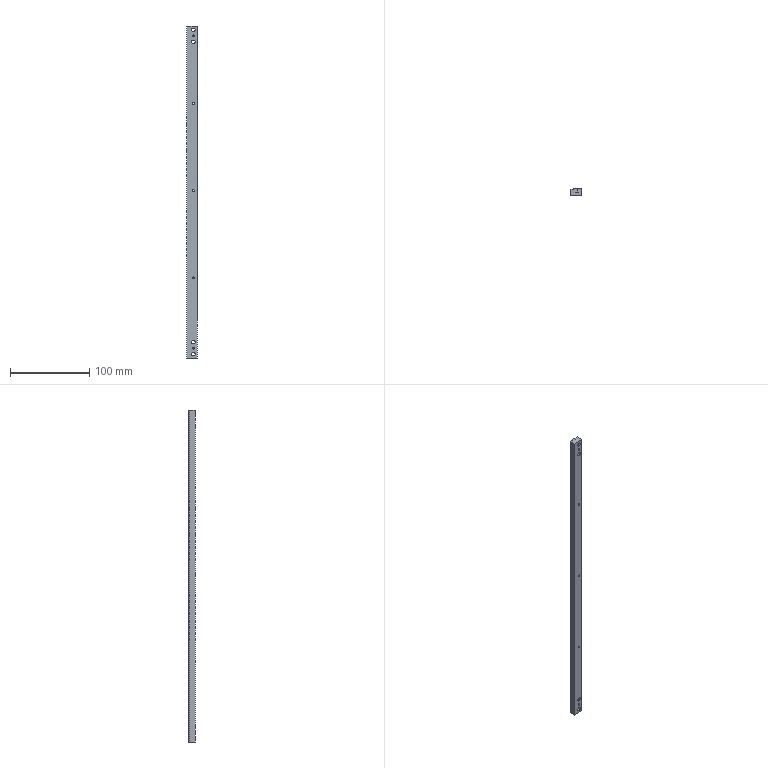Part | STEP file | 11-FG-B00611 | 1 solid | 47 faces | box 13.5 x 8.4 x 419 mm | volume 44557 mm3 | cylinder 30 | plane 13 | cone 4 | commonest cylinder face diameters 2.5 x14 4.5 x8 8 x8
STEP:
#1=CARTESIAN_POINT('',(8.5,0.,209.75));
#2=VERTEX_POINT('',#1);
#3=CARTESIAN_POINT('',(8.5,0.,212.25));
#4=VERTEX_POINT('',#3);
#5=CARTESIAN_POINT('',(8.5,0.,211.));
#6=DIRECTION('',(0.,1.,0.));
#7=DIRECTION('',(0.,0.,1.));
#8=AXIS2_PLACEMENT_3D('',#5,#6,#7);
#9=CIRCLE('',#8,1.25);
#10=EDGE_CURVE('',#2,#4,#9,.T.);
#11=ORIENTED_EDGE('',*,*,#10,.F.);
#12=CARTESIAN_POINT('',(8.5,8.4,209.75));
#13=VERTEX_POINT('',#12);
#14=CARTESIAN_POINT('',(8.5,8.,209.75));
#15=DIRECTION('',(0.,1.,0.));
#16=VECTOR('',#15,1000.);
#17=LINE('',#14,#16);
#18=EDGE_CURVE('',#2,#13,#17,.T.);
#19=ORIENTED_EDGE('',*,*,#18,.T.);
#20=CARTESIAN_POINT('',(8.5,8.4,212.25));
#21=VERTEX_POINT('',#20);
#22=CARTESIAN_POINT('',(8.5,8.4,211.));
#23=DIRECTION('',(0.,1.,0.));
#24=DIRECTION('',(0.,0.,-1.));
#25=AXIS2_PLACEMENT_3D('',#22,#23,#24);
#26=CIRCLE('',#25,1.25);
#27=EDGE_CURVE('',#13,#21,#26,.T.);
#28=ORIENTED_EDGE('',*,*,#27,.T.);
#29=CARTESIAN_POINT('',(8.5,8.,212.25));
#30=DIRECTION('',(0.,1.,0.));
#31=VECTOR('',#30,1000.);
#32=LINE('',#29,#31);
#33=EDGE_CURVE('',#4,#21,#32,.T.);
#34=ORIENTED_EDGE('',*,*,#33,.F.);
#35=EDGE_LOOP('',(#11,#19,#28,#34));
#36=FACE_OUTER_BOUND('',#35,.T.);
#37=CARTESIAN_POINT('',(8.5,8.,211.));
#38=DIRECTION('',(0.,1.,0.));
#39=DIRECTION('',(0.,0.,1.));
#40=AXIS2_PLACEMENT_3D('',#37,#38,#39);
#41=CYLINDRICAL_SURFACE('',#40,1.25);
#42=ADVANCED_FACE('',(#36),#41,.F.);
#43=CARTESIAN_POINT('',(8.5,0.,319.75));
#44=VERTEX_POINT('',#43);
#45=CARTESIAN_POINT('',(8.5,0.,322.25));
#46=VERTEX_POINT('',#45);
#47=CARTESIAN_POINT('',(8.5,0.,321.));
#48=DIRECTION('',(0.,1.,0.));
#49=DIRECTION('',(0.,0.,1.));
#50=AXIS2_PLACEMENT_3D('',#47,#48,#49);
#51=CIRCLE('',#50,1.25);
#52=EDGE_CURVE('',#44,#46,#51,.T.);
#53=ORIENTED_EDGE('',*,*,#52,.F.);
#54=CARTESIAN_POINT('',(8.5,8.4,319.75));
#55=VERTEX_POINT('',#54);
#56=CARTESIAN_POINT('',(8.5,8.,319.75));
#57=DIRECTION('',(0.,1.,0.));
#58=VECTOR('',#57,1000.);
#59=LINE('',#56,#58);
#60=EDGE_CURVE('',#44,#55,#59,.T.);
#61=ORIENTED_EDGE('',*,*,#60,.T.);
#62=CARTESIAN_POINT('',(8.5,8.4,322.25));
#63=VERTEX_POINT('',#62);
#64=CARTESIAN_POINT('',(8.5,8.4,321.));
#65=DIRECTION('',(0.,1.,0.));
#66=DIRECTION('',(0.,0.,-1.));
#67=AXIS2_PLACEMENT_3D('',#64,#65,#66);
#68=CIRCLE('',#67,1.25);
#69=EDGE_CURVE('',#55,#63,#68,.T.);
#70=ORIENTED_EDGE('',*,*,#69,.T.);
#71=CARTESIAN_POINT('',(8.5,8.,322.25));
#72=DIRECTION('',(0.,1.,0.));
#73=VECTOR('',#72,1000.);
#74=LINE('',#71,#73);
#75=EDGE_CURVE('',#46,#63,#74,.T.);
#76=ORIENTED_EDGE('',*,*,#75,.F.);
#77=EDGE_LOOP('',(#53,#61,#70,#76));
#78=FACE_OUTER_BOUND('',#77,.T.);
#79=CARTESIAN_POINT('',(8.5,8.,321.));
#80=DIRECTION('',(0.,1.,0.));
#81=DIRECTION('',(0.,0.,1.));
#82=AXIS2_PLACEMENT_3D('',#79,#80,#81);
#83=CYLINDRICAL_SURFACE('',#82,1.25);
#84=ADVANCED_FACE('',(#78),#83,.F.);
#85=CARTESIAN_POINT('',(8.5,0.,99.75));
#86=VERTEX_POINT('',#85);
#87=CARTESIAN_POINT('',(8.5,0.,102.25));
#88=VERTEX_POINT('',#87);
#89=CARTESIAN_POINT('',(8.5,0.,101.));
#90=DIRECTION('',(0.,1.,0.));
#91=DIRECTION('',(0.,0.,1.));
#92=AXIS2_PLACEMENT_3D('',#89,#90,#91);
#93=CIRCLE('',#92,1.25);
#94=EDGE_CURVE('',#86,#88,#93,.T.);
#95=ORIENTED_EDGE('',*,*,#94,.F.);
#96=CARTESIAN_POINT('',(8.5,8.4,99.75));
#97=VERTEX_POINT('',#96);
#98=CARTESIAN_POINT('',(8.5,8.,99.75));
#99=DIRECTION('',(0.,1.,0.));
#100=VECTOR('',#99,1000.);
#101=LINE('',#98,#100);
#102=EDGE_CURVE('',#86,#97,#101,.T.);
#103=ORIENTED_EDGE('',*,*,#102,.T.);
#104=CARTESIAN_POINT('',(8.5,8.4,102.25));
#105=VERTEX_POINT('',#104);
#106=CARTESIAN_POINT('',(8.5,8.4,101.));
#107=DIRECTION('',(0.,1.,0.));
#108=DIRECTION('',(0.,0.,-1.));
#109=AXIS2_PLACEMENT_3D('',#106,#107,#108);
#110=CIRCLE('',#109,1.25);
#111=EDGE_CURVE('',#97,#105,#110,.T.);
#112=ORIENTED_EDGE('',*,*,#111,.T.);
#113=CARTESIAN_POINT('',(8.5,8.,102.25));
#114=DIRECTION('',(0.,1.,0.));
#115=VECTOR('',#114,1000.);
#116=LINE('',#113,#115);
#117=EDGE_CURVE('',#88,#105,#116,.T.);
#118=ORIENTED_EDGE('',*,*,#117,.F.);
#119=EDGE_LOOP('',(#95,#103,#112,#118));
#120=FACE_OUTER_BOUND('',#119,.T.);
#121=CARTESIAN_POINT('',(8.5,8.,101.));
#122=DIRECTION('',(0.,1.,0.));
#123=DIRECTION('',(0.,0.,1.));
#124=AXIS2_PLACEMENT_3D('',#121,#122,#123);
#125=CYLINDRICAL_SURFACE('',#124,1.25);
#126=ADVANCED_FACE('',(#120),#125,.F.);
#127=CARTESIAN_POINT('',(8.5,0.,11.25));
#128=VERTEX_POINT('',#127);
#129=CARTESIAN_POINT('',(8.5,0.,13.75));
#130=VERTEX_POINT('',#129);
#131=CARTESIAN_POINT('',(8.5,0.,12.5));
#132=DIRECTION('',(0.,1.,0.));
#133=DIRECTION('',(0.,0.,1.));
#134=AXIS2_PLACEMENT_3D('',#131,#132,#133);
#135=CIRCLE('',#134,1.25);
#136=EDGE_CURVE('',#128,#130,#135,.T.);
#137=ORIENTED_EDGE('',*,*,#136,.F.);
#138=CARTESIAN_POINT('',(8.5,8.4,11.25));
#139=VERTEX_POINT('',#138);
#140=CARTESIAN_POINT('',(8.5,8.,11.25));
#141=DIRECTION('',(0.,1.,0.));
#142=VECTOR('',#141,1000.);
#143=LINE('',#140,#142);
#144=EDGE_CURVE('',#128,#139,#143,.T.);
#145=ORIENTED_EDGE('',*,*,#144,.T.);
#146=CARTESIAN_POINT('',(8.5,8.4,13.75));
#147=VERTEX_POINT('',#146);
#148=CARTESIAN_POINT('',(8.5,8.4,12.5));
#149=DIRECTION('',(0.,1.,0.));
#150=DIRECTION('',(0.,0.,-1.));
#151=AXIS2_PLACEMENT_3D('',#148,#149,#150);
#152=CIRCLE('',#151,1.25);
#153=EDGE_CURVE('',#139,#147,#152,.T.);
#154=ORIENTED_EDGE('',*,*,#153,.T.);
#155=CARTESIAN_POINT('',(8.5,8.,13.75));
#156=DIRECTION('',(0.,1.,0.));
#157=VECTOR('',#156,1000.);
#158=LINE('',#155,#157);
#159=EDGE_CURVE('',#130,#147,#158,.T.);
#160=ORIENTED_EDGE('',*,*,#159,.F.);
#161=EDGE_LOOP('',(#137,#145,#154,#160));
#162=FACE_OUTER_BOUND('',#161,.T.);
#163=CARTESIAN_POINT('',(8.5,8.,12.5));
#164=DIRECTION('',(0.,1.,0.));
#165=DIRECTION('',(0.,0.,1.));
#166=AXIS2_PLACEMENT_3D('',#163,#164,#165);
#167=CYLINDRICAL_SURFACE('',#166,1.25);
#168=ADVANCED_FACE('',(#162),#167,.F.);
#169=CARTESIAN_POINT('',(8.5,0.,405.25));
#170=VERTEX_POINT('',#169);
#171=CARTESIAN_POINT('',(8.5,0.,407.75));
#172=VERTEX_POINT('',#171);
#173=CARTESIAN_POINT('',(8.5,0.,406.5));
#174=DIRECTION('',(0.,1.,0.));
#175=DIRECTION('',(0.,0.,1.));
#176=AXIS2_PLACEMENT_3D('',#173,#174,#175);
#177=CIRCLE('',#176,1.25);
#178=EDGE_CURVE('',#170,#172,#177,.T.);
#179=ORIENTED_EDGE('',*,*,#178,.F.);
#180=CARTESIAN_POINT('',(8.5,8.4,405.25));
#181=VERTEX_POINT('',#180);
#182=CARTESIAN_POINT('',(8.5,8.,405.25));
#183=DIRECTION('',(0.,1.,0.));
#184=VECTOR('',#183,1000.);
#185=LINE('',#182,#184);
#186=EDGE_CURVE('',#170,#181,#185,.T.);
#187=ORIENTED_EDGE('',*,*,#186,.T.);
#188=CARTESIAN_POINT('',(8.5,8.4,407.75));
#189=VERTEX_POINT('',#188);
#190=CARTESIAN_POINT('',(8.5,8.4,406.5));
#191=DIRECTION('',(0.,1.,0.));
#192=DIRECTION('',(0.,0.,-1.));
#193=AXIS2_PLACEMENT_3D('',#190,#191,#192);
#194=CIRCLE('',#193,1.25);
#195=EDGE_CURVE('',#181,#189,#194,.T.);
#196=ORIENTED_EDGE('',*,*,#195,.T.);
#197=CARTESIAN_POINT('',(8.5,8.,407.75));
#198=DIRECTION('',(0.,1.,0.));
#199=VECTOR('',#198,1000.);
#200=LINE('',#197,#199);
#201=EDGE_CURVE('',#172,#189,#200,.T.);
#202=ORIENTED_EDGE('',*,*,#201,.F.);
#203=EDGE_LOOP('',(#179,#187,#196,#202));
#204=FACE_OUTER_BOUND('',#203,.T.);
#205=CARTESIAN_POINT('',(8.5,8.,406.5));
#206=DIRECTION('',(0.,1.,0.));
#207=DIRECTION('',(0.,0.,1.));
#208=AXIS2_PLACEMENT_3D('',#205,#206,#207);
#209=CYLINDRICAL_SURFACE('',#208,1.25);
#210=ADVANCED_FACE('',(#204),#209,.F.);
#211=CARTESIAN_POINT('',(8.5,3.6,410.));
#212=VERTEX_POINT('',#211);
#213=CARTESIAN_POINT('',(8.5,3.6,418.));
#214=VERTEX_POINT('',#213);
#215=CARTESIAN_POINT('',(8.5,3.6,414.));
#216=DIRECTION('',(0.,1.,0.));
#217=DIRECTION('',(0.,0.,1.));
#218=AXIS2_PLACEMENT_3D('',#215,#216,#217);
#219=CIRCLE('',#218,4.);
#220=EDGE_CURVE('',#212,#214,#219,.T.);
#221=ORIENTED_EDGE('',*,*,#220,.F.);
#222=CARTESIAN_POINT('',(8.5,8.4,410.));
#223=VERTEX_POINT('',#222);
#224=CARTESIAN_POINT('',(8.5,8.,410.));
#225=DIRECTION('',(0.,1.,0.));
#226=VECTOR('',#225,1000.);
#227=LINE('',#224,#226);
#228=EDGE_CURVE('',#212,#223,#227,.T.);
#229=ORIENTED_EDGE('',*,*,#228,.T.);
#230=CARTESIAN_POINT('',(8.5,8.4,418.));
#231=VERTEX_POINT('',#230);
#232=CARTESIAN_POINT('',(8.5,8.4,414.));
#233=DIRECTION('',(0.,1.,0.));
#234=DIRECTION('',(0.,0.,-1.));
#235=AXIS2_PLACEMENT_3D('',#232,#233,#234);
#236=CIRCLE('',#235,4.);
#237=EDGE_CURVE('',#223,#231,#236,.T.);
#238=ORIENTED_EDGE('',*,*,#237,.T.);
#239=CARTESIAN_POINT('',(8.5,8.,418.));
#240=DIRECTION('',(0.,1.,0.));
#241=VECTOR('',#240,1000.);
#242=LINE('',#239,#241);
#243=EDGE_CURVE('',#214,#231,#242,.T.);
#244=ORIENTED_EDGE('',*,*,#243,.F.);
#245=EDGE_LOOP('',(#221,#229,#238,#244));
#246=FACE_OUTER_BOUND('',#245,.T.);
#247=CARTESIAN_POINT('',(8.5,8.,414.));
#248=DIRECTION('',(0.,1.,0.));
#249=DIRECTION('',(0.,0.,1.));
#250=AXIS2_PLACEMENT_3D('',#247,#248,#249);
#251=CYLINDRICAL_SURFACE('',#250,4.);
#252=ADVANCED_FACE('',(#246),#251,.F.);
#253=CARTESIAN_POINT('',(8.5,0.,411.75));
#254=VERTEX_POINT('',#253);
#255=CARTESIAN_POINT('',(8.5,0.,416.25));
#256=VERTEX_POINT('',#255);
#257=CARTESIAN_POINT('',(8.5,0.,414.));
#258=DIRECTION('',(0.,1.,0.));
#259=DIRECTION('',(0.,0.,1.));
#260=AXIS2_PLACEMENT_3D('',#257,#258,#259);
#261=CIRCLE('',#260,2.25);
#262=EDGE_CURVE('',#254,#256,#261,.T.);
#263=ORIENTED_EDGE('',*,*,#262,.F.);
#264=CARTESIAN_POINT('',(8.5,3.6,411.75));
#265=VERTEX_POINT('',#264);
#266=CARTESIAN_POINT('',(8.5,8.,411.75));
#267=DIRECTION('',(0.,1.,0.));
#268=VECTOR('',#267,1000.);
#269=LINE('',#266,#268);
#270=EDGE_CURVE('',#254,#265,#269,.T.);
#271=ORIENTED_EDGE('',*,*,#270,.T.);
#272=CARTESIAN_POINT('',(8.5,3.6,416.25));
#273=VERTEX_POINT('',#272);
#274=CARTESIAN_POINT('',(8.5,3.6,414.));
#275=DIRECTION('',(0.,1.,0.));
#276=DIRECTION('',(0.,0.,1.));
#277=AXIS2_PLACEMENT_3D('',#274,#275,#276);
#278=CIRCLE('',#277,2.25);
#279=EDGE_CURVE('',#265,#273,#278,.T.);
#280=ORIENTED_EDGE('',*,*,#279,.T.);
#281=CARTESIAN_POINT('',(8.5,8.,416.25));
#282=DIRECTION('',(0.,1.,0.));
#283=VECTOR('',#282,1000.);
#284=LINE('',#281,#283);
#285=EDGE_CURVE('',#256,#273,#284,.T.);
#286=ORIENTED_EDGE('',*,*,#285,.F.);
#287=EDGE_LOOP('',(#263,#271,#280,#286));
#288=FACE_OUTER_BOUND('',#287,.T.);
#289=CARTESIAN_POINT('',(8.5,8.,414.));
#290=DIRECTION('',(0.,1.,0.));
#291=DIRECTION('',(0.,0.,1.));
#292=AXIS2_PLACEMENT_3D('',#289,#290,#291);
#293=CYLINDRICAL_SURFACE('',#292,2.25);
#294=ADVANCED_FACE('',(#288),#293,.F.);
#295=CARTESIAN_POINT('',(8.5,3.6,395.));
#296=VERTEX_POINT('',#295);
#297=CARTESIAN_POINT('',(8.5,3.6,403.));
#298=VERTEX_POINT('',#297);
#299=CARTESIAN_POINT('',(8.5,3.6,399.));
#300=DIRECTION('',(0.,1.,0.));
#301=DIRECTION('',(0.,0.,1.));
#302=AXIS2_PLACEMENT_3D('',#299,#300,#301);
#303=CIRCLE('',#302,4.);
#304=EDGE_CURVE('',#296,#298,#303,.T.);
#305=ORIENTED_EDGE('',*,*,#304,.F.);
#306=CARTESIAN_POINT('',(8.5,8.4,395.));
#307=VERTEX_POINT('',#306);
#308=CARTESIAN_POINT('',(8.5,8.,395.));
#309=DIRECTION('',(0.,1.,0.));
#310=VECTOR('',#309,1000.);
#311=LINE('',#308,#310);
#312=EDGE_CURVE('',#296,#307,#311,.T.);
#313=ORIENTED_EDGE('',*,*,#312,.T.);
#314=CARTESIAN_POINT('',(8.5,8.4,403.));
#315=VERTEX_POINT('',#314);
#316=CARTESIAN_POINT('',(8.5,8.4,399.));
#317=DIRECTION('',(0.,1.,0.));
#318=DIRECTION('',(0.,0.,-1.));
#319=AXIS2_PLACEMENT_3D('',#316,#317,#318);
#320=CIRCLE('',#319,4.);
#321=EDGE_CURVE('',#307,#315,#320,.T.);
#322=ORIENTED_EDGE('',*,*,#321,.T.);
#323=CARTESIAN_POINT('',(8.5,8.,403.));
#324=DIRECTION('',(0.,1.,0.));
#325=VECTOR('',#324,1000.);
#326=LINE('',#323,#325);
#327=EDGE_CURVE('',#298,#315,#326,.T.);
#328=ORIENTED_EDGE('',*,*,#327,.F.);
#329=EDGE_LOOP('',(#305,#313,#322,#328));
#330=FACE_OUTER_BOUND('',#329,.T.);
#331=CARTESIAN_POINT('',(8.5,8.,399.));
#332=DIRECTION('',(0.,1.,0.));
#333=DIRECTION('',(0.,0.,1.));
#334=AXIS2_PLACEMENT_3D('',#331,#332,#333);
#335=CYLINDRICAL_SURFACE('',#334,4.);
#336=ADVANCED_FACE('',(#330),#335,.F.);
#337=CARTESIAN_POINT('',(8.5,0.,396.75));
#338=VERTEX_POINT('',#337);
#339=CARTESIAN_POINT('',(8.5,0.,401.25));
#340=VERTEX_POINT('',#339);
#341=CARTESIAN_POINT('',(8.5,0.,399.));
#342=DIRECTION('',(0.,1.,0.));
#343=DIRECTION('',(0.,0.,1.));
#344=AXIS2_PLACEMENT_3D('',#341,#342,#343);
#345=CIRCLE('',#344,2.25);
#346=EDGE_CURVE('',#338,#340,#345,.T.);
#347=ORIENTED_EDGE('',*,*,#346,.F.);
#348=CARTESIAN_POINT('',(8.5,3.6,396.75));
#349=VERTEX_POINT('',#348);
#350=CARTESIAN_POINT('',(8.5,8.,396.75));
#351=DIRECTION('',(0.,1.,0.));
#352=VECTOR('',#351,1000.);
#353=LINE('',#350,#352);
#354=EDGE_CURVE('',#338,#349,#353,.T.);
#355=ORIENTED_EDGE('',*,*,#354,.T.);
#356=CARTESIAN_POINT('',(8.5,3.6,401.25));
#357=VERTEX_POINT('',#356);
#358=CARTESIAN_POINT('',(8.5,3.6,399.));
#359=DIRECTION('',(0.,1.,0.));
#360=DIRECTION('',(0.,0.,1.));
#361=AXIS2_PLACEMENT_3D('',#358,#359,#360);
#362=CIRCLE('',#361,2.25);
#363=EDGE_CURVE('',#349,#357,#362,.T.);
#364=ORIENTED_EDGE('',*,*,#363,.T.);
#365=CARTESIAN_POINT('',(8.5,8.,401.25));
#366=DIRECTION('',(0.,1.,0.));
#367=VECTOR('',#366,1000.);
#368=LINE('',#365,#367);
#369=EDGE_CURVE('',#340,#357,#368,.T.);
#370=ORIENTED_EDGE('',*,*,#369,.F.);
#371=EDGE_LOOP('',(#347,#355,#364,#370));
#372=FACE_OUTER_BOUND('',#371,.T.);
#373=CARTESIAN_POINT('',(8.5,8.,399.));
#374=DIRECTION('',(0.,1.,0.));
#375=DIRECTION('',(0.,0.,1.));
#376=AXIS2_PLACEMENT_3D('',#373,#374,#375);
#377=CYLINDRICAL_SURFACE('',#376,2.25);
#378=ADVANCED_FACE('',(#372),#377,.F.);
#379=CARTESIAN_POINT('',(6.,4.,49.75));
#380=VERTEX_POINT('',#379);
#381=CARTESIAN_POINT('',(6.,4.,47.25));
#382=VERTEX_POINT('',#381);
#383=CARTESIAN_POINT('',(6.,4.,48.5));
#384=DIRECTION('',(1.,0.,0.));
#385=DIRECTION('',(0.,0.,-1.));
#386=AXIS2_PLACEMENT_3D('',#383,#384,#385);
#387=CIRCLE('',#386,1.25);
#388=EDGE_CURVE('',#380,#382,#387,.T.);
#389=ORIENTED_EDGE('',*,*,#388,.F.);
#390=CARTESIAN_POINT('',(13.5,4.,49.75));
#391=VERTEX_POINT('',#390);
#392=CARTESIAN_POINT('',(13.5,4.,49.75));
#393=DIRECTION('',(1.,0.,0.));
#394=VECTOR('',#393,1000.);
#395=LINE('',#392,#394);
#396=EDGE_CURVE('',#380,#391,#395,.T.);
#397=ORIENTED_EDGE('',*,*,#396,.T.);
#398=CARTESIAN_POINT('',(13.5,4.,47.25));
#399=VERTEX_POINT('',#398);
#400=CARTESIAN_POINT('',(13.5,4.,48.5));
#401=DIRECTION('',(1.,0.,0.));
#402=DIRECTION('',(0.,0.,-1.));
#403=AXIS2_PLACEMENT_3D('',#400,#401,#402);
#404=CIRCLE('',#403,1.25);
#405=EDGE_CURVE('',#391,#399,#404,.T.);
#406=ORIENTED_EDGE('',*,*,#405,.T.);
#407=CARTESIAN_POINT('',(13.5,4.,47.25));
#408=DIRECTION('',(1.,0.,0.));
#409=VECTOR('',#408,1000.);
#410=LINE('',#407,#409);
#411=EDGE_CURVE('',#382,#399,#410,.T.);
#412=ORIENTED_EDGE('',*,*,#411,.F.);
#413=EDGE_LOOP('',(#389,#397,#406,#412));
#414=FACE_OUTER_BOUND('',#413,.T.);
#415=CARTESIAN_POINT('',(13.5,4.,48.5));
#416=DIRECTION('',(1.,0.,0.));
#417=DIRECTION('',(0.,0.,-1.));
#418=AXIS2_PLACEMENT_3D('',#415,#416,#417);
#419=CYLINDRICAL_SURFACE('',#418,1.25);
#420=ADVANCED_FACE('',(#414),#419,.F.);
#421=CARTESIAN_POINT('',(5.249,4.,48.5));
#422=VERTEX_POINT('',#421);
#423=CARTESIAN_POINT('',(6.,4.,47.25));
#424=DIRECTION('',(0.515,0.,-0.8572));
#425=VECTOR('',#424,1000.);
#426=LINE('',#423,#425);
#427=EDGE_CURVE('',#422,#382,#426,.T.);
#428=ORIENTED_EDGE('',*,*,#427,.F.);
#429=CARTESIAN_POINT('',(6.,4.,49.75));
#430=DIRECTION('',(0.515,0.,0.8572));
#431=VECTOR('',#430,1000.);
#432=LINE('',#429,#431);
#433=EDGE_CURVE('',#422,#380,#432,.T.);
#434=ORIENTED_EDGE('',*,*,#433,.T.);
#435=ORIENTED_EDGE('',*,*,#388,.T.);
#436=EDGE_LOOP('',(#428,#434,#435));
#437=FACE_OUTER_BOUND('',#436,.T.);
#438=CARTESIAN_POINT('',(6.,4.,48.5));
#439=DIRECTION('',(1.,0.,0.));
#440=DIRECTION('',(0.,0.,-1.));
#441=AXIS2_PLACEMENT_3D('',#438,#439,#440);
#442=CONICAL_SURFACE('',#441,1.25,1.03);
#443=ADVANCED_FACE('',(#437),#442,.F.);
#444=CARTESIAN_POINT('',(6.,4.,42.75));
#445=VERTEX_POINT('',#444);
#446=CARTESIAN_POINT('',(6.,4.,40.25));
#447=VERTEX_POINT('',#446);
#448=CARTESIAN_POINT('',(6.,4.,41.5));
#449=DIRECTION('',(1.,0.,0.));
#450=DIRECTION('',(0.,0.,-1.));
#451=AXIS2_PLACEMENT_3D('',#448,#449,#450);
#452=CIRCLE('',#451,1.25);
#453=EDGE_CURVE('',#445,#447,#452,.T.);
#454=ORIENTED_EDGE('',*,*,#453,.F.);
#455=CARTESIAN_POINT('',(13.5,4.,42.75));
#456=VERTEX_POINT('',#455);
#457=CARTESIAN_POINT('',(13.5,4.,42.75));
#458=DIRECTION('',(1.,0.,0.));
#459=VECTOR('',#458,1000.);
#460=LINE('',#457,#459);
#461=EDGE_CURVE('',#445,#456,#460,.T.);
#462=ORIENTED_EDGE('',*,*,#461,.T.);
#463=CARTESIAN_POINT('',(13.5,4.,40.25));
#464=VERTEX_POINT('',#463);
#465=CARTESIAN_POINT('',(13.5,4.,41.5));
#466=DIRECTION('',(1.,0.,0.));
#467=DIRECTION('',(0.,0.,-1.));
#468=AXIS2_PLACEMENT_3D('',#465,#466,#467);
#469=CIRCLE('',#468,1.25);
#470=EDGE_CURVE('',#456,#464,#469,.T.);
#471=ORIENTED_EDGE('',*,*,#470,.T.);
#472=CARTESIAN_POINT('',(13.5,4.,40.25));
#473=DIRECTION('',(1.,0.,0.));
#474=VECTOR('',#473,1000.);
#475=LINE('',#472,#474);
#476=EDGE_CURVE('',#447,#464,#475,.T.);
#477=ORIENTED_EDGE('',*,*,#476,.F.);
#478=EDGE_LOOP('',(#454,#462,#471,#477));
#479=FACE_OUTER_BOUND('',#478,.T.);
#480=CARTESIAN_POINT('',(13.5,4.,41.5));
#481=DIRECTION('',(1.,0.,0.));
#482=DIRECTION('',(0.,0.,-1.));
#483=AXIS2_PLACEMENT_3D('',#480,#481,#482);
#484=CYLINDRICAL_SURFACE('',#483,1.25);
#485=ADVANCED_FACE('',(#479),#484,.F.);
#486=CARTESIAN_POINT('',(5.249,4.,41.5));
#487=VERTEX_POINT('',#486);
#488=CARTESIAN_POINT('',(6.,4.,40.25));
#489=DIRECTION('',(0.515,0.,-0.8572));
#490=VECTOR('',#489,1000.);
#491=LINE('',#488,#490);
#492=EDGE_CURVE('',#487,#447,#491,.T.);
#493=ORIENTED_EDGE('',*,*,#492,.F.);
#494=CARTESIAN_POINT('',(6.,4.,42.75));
#495=DIRECTION('',(0.515,0.,0.8572));
#496=VECTOR('',#495,1000.);
#497=LINE('',#494,#496);
#498=EDGE_CURVE('',#487,#445,#497,.T.);
#499=ORIENTED_EDGE('',*,*,#498,.T.);
#500=ORIENTED_EDGE('',*,*,#453,.T.);
#501=EDGE_LOOP('',(#493,#499,#500));
#502=FACE_OUTER_BOUND('',#501,.T.);
#503=CARTESIAN_POINT('',(6.,4.,41.5));
#504=DIRECTION('',(1.,0.,0.));
#505=DIRECTION('',(0.,0.,-1.));
#506=AXIS2_PLACEMENT_3D('',#503,#504,#505);
#507=CONICAL_SURFACE('',#506,1.25,1.03);
#508=ADVANCED_FACE('',(#502),#507,.F.);
#509=CARTESIAN_POINT('',(8.5,3.4,16.));
#510=VERTEX_POINT('',#509);
#511=CARTESIAN_POINT('',(8.5,3.4,24.));
#512=VERTEX_POINT('',#511);
#513=CARTESIAN_POINT('',(8.5,3.4,20.));
#514=DIRECTION('',(0.,1.,0.));
#515=DIRECTION('',(0.,0.,1.));
#516=AXIS2_PLACEMENT_3D('',#513,#514,#515);
#517=CIRCLE('',#516,4.);
#518=EDGE_CURVE('',#510,#512,#517,.T.);
#519=ORIENTED_EDGE('',*,*,#518,.F.);
#520=CARTESIAN_POINT('',(8.5,8.4,16.));
#521=VERTEX_POINT('',#520);
#522=CARTESIAN_POINT('',(8.5,8.,16.));
#523=DIRECTION('',(0.,1.,0.));
#524=VECTOR('',#523,1000.);
#525=LINE('',#522,#524);
#526=EDGE_CURVE('',#510,#521,#525,.T.);
#527=ORIENTED_EDGE('',*,*,#526,.T.);
#528=CARTESIAN_POINT('',(8.5,8.4,24.));
#529=VERTEX_POINT('',#528);
#530=CARTESIAN_POINT('',(8.5,8.4,20.));
#531=DIRECTION('',(0.,1.,0.));
#532=DIRECTION('',(0.,0.,-1.));
#533=AXIS2_PLACEMENT_3D('',#530,#531,#532);
#534=CIRCLE('',#533,4.);
#535=EDGE_CURVE('',#521,#529,#534,.T.);
#536=ORIENTED_EDGE('',*,*,#535,.T.);
#537=CARTESIAN_POINT('',(8.5,8.,24.));
#538=DIRECTION('',(0.,1.,0.));
#539=VECTOR('',#538,1000.);
#540=LINE('',#537,#539);
#541=EDGE_CURVE('',#512,#529,#540,.T.);
#542=ORIENTED_EDGE('',*,*,#541,.F.);
#543=EDGE_LOOP('',(#519,#527,#536,#542));
#544=FACE_OUTER_BOUND('',#543,.T.);
#545=CARTESIAN_POINT('',(8.5,8.,20.));
#546=DIRECTION('',(0.,1.,0.));
#547=DIRECTION('',(0.,0.,1.));
#548=AXIS2_PLACEMENT_3D('',#545,#546,#547);
#549=CYLINDRICAL_SURFACE('',#548,4.);
#550=ADVANCED_FACE('',(#544),#549,.F.);
#551=CARTESIAN_POINT('',(8.5,0.,17.75));
#552=VERTEX_POINT('',#551);
#553=CARTESIAN_POINT('',(8.5,0.,22.25));
#554=VERTEX_POINT('',#553);
#555=CARTESIAN_POINT('',(8.5,0.,20.));
#556=DIRECTION('',(0.,1.,0.));
#557=DIRECTION('',(0.,0.,1.));
#558=AXIS2_PLACEMENT_3D('',#555,#556,#557);
#559=CIRCLE('',#558,2.25);
#560=EDGE_CURVE('',#552,#554,#559,.T.);
#561=ORIENTED_EDGE('',*,*,#560,.F.);
#562=CARTESIAN_POINT('',(8.5,3.4,17.75));
#563=VERTEX_POINT('',#562);
#564=CARTESIAN_POINT('',(8.5,8.,17.75));
#565=DIRECTION('',(0.,1.,0.));
#566=VECTOR('',#565,1000.);
#567=LINE('',#564,#566);
#568=EDGE_CURVE('',#552,#563,#567,.T.);
#569=ORIENTED_EDGE('',*,*,#568,.T.);
#570=CARTESIAN_POINT('',(8.5,3.4,22.25));
#571=VERTEX_POINT('',#570);
#572=CARTESIAN_POINT('',(8.5,3.4,20.));
#573=DIRECTION('',(0.,1.,0.));
#574=DIRECTION('',(0.,0.,1.));
#575=AXIS2_PLACEMENT_3D('',#572,#573,#574);
#576=CIRCLE('',#575,2.25);
#577=EDGE_CURVE('',#563,#571,#576,.T.);
#578=ORIENTED_EDGE('',*,*,#577,.T.);
#579=CARTESIAN_POINT('',(8.5,8.,22.25));
#580=DIRECTION('',(0.,1.,0.));
#581=VECTOR('',#580,1000.);
#582=LINE('',#579,#581);
#583=EDGE_CURVE('',#554,#571,#582,.T.);
#584=ORIENTED_EDGE('',*,*,#583,.F.);
#585=EDGE_LOOP('',(#561,#569,#578,#584));
#586=FACE_OUTER_BOUND('',#585,.T.);
#587=CARTESIAN_POINT('',(8.5,8.,20.));
#588=DIRECTION('',(0.,1.,0.));
#589=DIRECTION('',(0.,0.,1.));
#590=AXIS2_PLACEMENT_3D('',#587,#588,#589);
#591=CYLINDRICAL_SURFACE('',#590,2.25);
#592=ADVANCED_FACE('',(#586),#591,.F.);
#593=CARTESIAN_POINT('',(8.5,3.4,1.));
#594=VERTEX_POINT('',#593);
#595=CARTESIAN_POINT('',(8.5,3.4,9.));
#596=VERTEX_POINT('',#595);
#597=CARTESIAN_POINT('',(8.5,3.4,5.));
#598=DIRECTION('',(0.,1.,0.));
#599=DIRECTION('',(0.,0.,1.));
#600=AXIS2_PLACEMENT_3D('',#597,#598,#599);
#601=CIRCLE('',#600,4.);
#602=EDGE_CURVE('',#594,#596,#601,.T.);
#603=ORIENTED_EDGE('',*,*,#602,.F.);
#604=CARTESIAN_POINT('',(8.5,8.4,1.));
#605=VERTEX_POINT('',#604);
#606=CARTESIAN_POINT('',(8.5,8.,1.));
#607=DIRECTION('',(0.,1.,0.));
#608=VECTOR('',#607,1000.);
#609=LINE('',#606,#608);
#610=EDGE_CURVE('',#594,#605,#609,.T.);
#611=ORIENTED_EDGE('',*,*,#610,.T.);
#612=CARTESIAN_POINT('',(8.5,8.4,9.));
#613=VERTEX_POINT('',#612);
#614=CARTESIAN_POINT('',(8.5,8.4,5.));
#615=DIRECTION('',(0.,1.,0.));
#616=DIRECTION('',(0.,0.,-1.));
#617=AXIS2_PLACEMENT_3D('',#614,#615,#616);
#618=CIRCLE('',#617,4.);
#619=EDGE_CURVE('',#605,#613,#618,.T.);
#620=ORIENTED_EDGE('',*,*,#619,.T.);
#621=CARTESIAN_POINT('',(8.5,8.,9.));
#622=DIRECTION('',(0.,1.,0.));
#623=VECTOR('',#622,1000.);
#624=LINE('',#621,#623);
#625=EDGE_CURVE('',#596,#613,#624,.T.);
#626=ORIENTED_EDGE('',*,*,#625,.F.);
#627=EDGE_LOOP('',(#603,#611,#620,#626));
#628=FACE_OUTER_BOUND('',#627,.T.);
#629=CARTESIAN_POINT('',(8.5,8.,5.));
#630=DIRECTION('',(0.,1.,0.));
#631=DIRECTION('',(0.,0.,1.));
#632=AXIS2_PLACEMENT_3D('',#629,#630,#631);
#633=CYLINDRICAL_SURFACE('',#632,4.);
#634=ADVANCED_FACE('',(#628),#633,.F.);
#635=CARTESIAN_POINT('',(8.5,0.,2.75));
#636=VERTEX_POINT('',#635);
#637=CARTESIAN_POINT('',(8.5,0.,7.25));
#638=VERTEX_POINT('',#637);
#639=CARTESIAN_POINT('',(8.5,0.,5.));
#640=DIRECTION('',(0.,1.,0.));
#641=DIRECTION('',(0.,0.,1.));
#642=AXIS2_PLACEMENT_3D('',#639,#640,#641);
#643=CIRCLE('',#642,2.25);
#644=EDGE_CURVE('',#636,#638,#643,.T.);
#645=ORIENTED_EDGE('',*,*,#644,.F.);
#646=CARTESIAN_POINT('',(8.5,3.4,2.75));
#647=VERTEX_POINT('',#646);
#648=CARTESIAN_POINT('',(8.5,8.,2.75));
#649=DIRECTION('',(0.,1.,0.));
#650=VECTOR('',#649,1000.);
#651=LINE('',#648,#650);
#652=EDGE_CURVE('',#636,#647,#651,.T.);
#653=ORIENTED_EDGE('',*,*,#652,.T.);
#654=CARTESIAN_POINT('',(8.5,3.4,7.25));
#655=VERTEX_POINT('',#654);
#656=CARTESIAN_POINT('',(8.5,3.4,5.));
#657=DIRECTION('',(0.,1.,0.));
#658=DIRECTION('',(0.,0.,1.));
#659=AXIS2_PLACEMENT_3D('',#656,#657,#658);
#660=CIRCLE('',#659,2.25);
#661=EDGE_CURVE('',#647,#655,#660,.T.);
#662=ORIENTED_EDGE('',*,*,#661,.T.);
#663=CARTESIAN_POINT('',(8.5,8.,7.25));
#664=DIRECTION('',(0.,1.,0.));
#665=VECTOR('',#664,1000.);
#666=LINE('',#663,#665);
#667=EDGE_CURVE('',#638,#655,#666,.T.);
#668=ORIENTED_EDGE('',*,*,#667,.F.);
#669=EDGE_LOOP('',(#645,#653,#662,#668));
#670=FACE_OUTER_BOUND('',#669,.T.);
#671=CARTESIAN_POINT('',(8.5,8.,5.));
#672=DIRECTION('',(0.,1.,0.));
#673=DIRECTION('',(0.,0.,1.));
#674=AXIS2_PLACEMENT_3D('',#671,#672,#673);
#675=CYLINDRICAL_SURFACE('',#674,2.25);
#676=ADVANCED_FACE('',(#670),#675,.F.);
#677=CARTESIAN_POINT('',(0.,7.4,0.));
#678=VERTEX_POINT('',#677);
#679=CARTESIAN_POINT('',(0.,0.,0.));
#680=VERTEX_POINT('',#679);
#681=CARTESIAN_POINT('',(0.,0.,0.));
#682=DIRECTION('',(0.,-1.,0.));
#683=VECTOR('',#682,1000.);
#684=LINE('',#681,#683);
#685=EDGE_CURVE('',#678,#680,#684,.T.);
#686=ORIENTED_EDGE('',*,*,#685,.T.);
#687=CARTESIAN_POINT('',(0.,0.,419.));
#688=VERTEX_POINT('',#687);
#689=CARTESIAN_POINT('',(0.,0.,400.));
#690=DIRECTION('',(0.,0.,-1.));
#691=VECTOR('',#690,1000.);
#692=LINE('',#689,#691);
#693=EDGE_CURVE('',#688,#680,#692,.T.);
#694=ORIENTED_EDGE('',*,*,#693,.F.);
#695=CARTESIAN_POINT('',(0.,7.4,419.));
#696=VERTEX_POINT('',#695);
#697=CARTESIAN_POINT('',(0.,0.,419.));
#698=DIRECTION('',(0.,-1.,0.));
#699=VECTOR('',#698,1000.);
#700=LINE('',#697,#699);
#701=EDGE_CURVE('',#696,#688,#700,.T.);
#702=ORIENTED_EDGE('',*,*,#701,.F.);
#703=CARTESIAN_POINT('',(0.,7.4,400.));
#704=DIRECTION('',(0.,0.,-1.));
#705=VECTOR('',#704,1000.);
#706=LINE('',#703,#705);
#707=EDGE_CURVE('',#696,#678,#706,.T.);
#708=ORIENTED_EDGE('',*,*,#707,.T.);
#709=EDGE_LOOP('',(#686,#694,#702,#708));
#710=FACE_OUTER_BOUND('',#709,.T.);
#711=CARTESIAN_POINT('',(0.,0.,400.));
#712=DIRECTION('',(1.,0.,0.));
#713=DIRECTION('',(0.,1.,0.));
#714=AXIS2_PLACEMENT_3D('',#711,#712,#713);
#715=PLANE('',#714);
#716=ADVANCED_FACE('',(#710),#715,.F.);
#717=CARTESIAN_POINT('',(8.5,0.,211.));
#718=DIRECTION('',(0.,1.,0.));
#719=DIRECTION('',(0.,0.,1.));
#720=AXIS2_PLACEMENT_3D('',#717,#718,#719);
#721=CIRCLE('',#720,1.25);
#722=EDGE_CURVE('',#4,#2,#721,.T.);
#723=ORIENTED_EDGE('',*,*,#722,.T.);
#724=ORIENTED_EDGE('',*,*,#10,.T.);
#725=EDGE_LOOP('',(#723,#724));
#726=FACE_BOUND('',#725,.T.);
#727=CARTESIAN_POINT('',(8.5,0.,321.));
#728=DIRECTION('',(0.,1.,0.));
#729=DIRECTION('',(0.,0.,1.));
#730=AXIS2_PLACEMENT_3D('',#727,#728,#729);
#731=CIRCLE('',#730,1.25);
#732=EDGE_CURVE('',#46,#44,#731,.T.);
#733=ORIENTED_EDGE('',*,*,#732,.T.);
#734=ORIENTED_EDGE('',*,*,#52,.T.);
#735=EDGE_LOOP('',(#733,#734));
#736=FACE_BOUND('',#735,.T.);
#737=CARTESIAN_POINT('',(8.5,0.,101.));
#738=DIRECTION('',(0.,1.,0.));
#739=DIRECTION('',(0.,0.,1.));
#740=AXIS2_PLACEMENT_3D('',#737,#738,#739);
#741=CIRCLE('',#740,1.25);
#742=EDGE_CURVE('',#88,#86,#741,.T.);
#743=ORIENTED_EDGE('',*,*,#742,.T.);
#744=ORIENTED_EDGE('',*,*,#94,.T.);
#745=EDGE_LOOP('',(#743,#744));
#746=FACE_BOUND('',#745,.T.);
#747=CARTESIAN_POINT('',(8.5,0.,12.5));
#748=DIRECTION('',(0.,1.,0.));
#749=DIRECTION('',(0.,0.,1.));
#750=AXIS2_PLACEMENT_3D('',#747,#748,#749);
#751=CIRCLE('',#750,1.25);
#752=EDGE_CURVE('',#130,#128,#751,.T.);
#753=ORIENTED_EDGE('',*,*,#752,.T.);
#754=ORIENTED_EDGE('',*,*,#136,.T.);
#755=EDGE_LOOP('',(#753,#754));
#756=FACE_BOUND('',#755,.T.);
#757=CARTESIAN_POINT('',(8.5,0.,406.5));
#758=DIRECTION('',(0.,1.,0.));
#759=DIRECTION('',(0.,0.,1.));
#760=AXIS2_PLACEMENT_3D('',#757,#758,#759);
#761=CIRCLE('',#760,1.25);
#762=EDGE_CURVE('',#172,#170,#761,.T.);
#763=ORIENTED_EDGE('',*,*,#762,.T.);
#764=ORIENTED_EDGE('',*,*,#178,.T.);
#765=EDGE_LOOP('',(#763,#764));
#766=FACE_BOUND('',#765,.T.);
#767=CARTESIAN_POINT('',(8.5,0.,414.));
#768=DIRECTION('',(0.,1.,0.));
#769=DIRECTION('',(0.,0.,1.));
#770=AXIS2_PLACEMENT_3D('',#767,#768,#769);
#771=CIRCLE('',#770,2.25);
#772=EDGE_CURVE('',#256,#254,#771,.T.);
#773=ORIENTED_EDGE('',*,*,#772,.T.);
#774=ORIENTED_EDGE('',*,*,#262,.T.);
#775=EDGE_LOOP('',(#773,#774));
#776=FACE_BOUND('',#775,.T.);
#777=CARTESIAN_POINT('',(8.5,0.,399.));
#778=DIRECTION('',(0.,1.,0.));
#779=DIRECTION('',(0.,0.,1.));
#780=AXIS2_PLACEMENT_3D('',#777,#778,#779);
#781=CIRCLE('',#780,2.25);
#782=EDGE_CURVE('',#340,#338,#781,.T.);
#783=ORIENTED_EDGE('',*,*,#782,.T.);
#784=ORIENTED_EDGE('',*,*,#346,.T.);
#785=EDGE_LOOP('',(#783,#784));
#786=FACE_BOUND('',#785,.T.);
#787=CARTESIAN_POINT('',(8.5,0.,20.));
#788=DIRECTION('',(0.,1.,0.));
#789=DIRECTION('',(0.,0.,1.));
#790=AXIS2_PLACEMENT_3D('',#787,#788,#789);
#791=CIRCLE('',#790,2.25);
#792=EDGE_CURVE('',#554,#552,#791,.T.);
#793=ORIENTED_EDGE('',*,*,#792,.T.);
#794=ORIENTED_EDGE('',*,*,#560,.T.);
#795=EDGE_LOOP('',(#793,#794));
#796=FACE_BOUND('',#795,.T.);
#797=CARTESIAN_POINT('',(8.5,0.,5.));
#798=DIRECTION('',(0.,1.,0.));
#799=DIRECTION('',(0.,0.,1.));
#800=AXIS2_PLACEMENT_3D('',#797,#798,#799);
#801=CIRCLE('',#800,2.25);
#802=EDGE_CURVE('',#638,#636,#801,.T.);
#803=ORIENTED_EDGE('',*,*,#802,.T.);
#804=ORIENTED_EDGE('',*,*,#644,.T.);
#805=EDGE_LOOP('',(#803,#804));
#806=FACE_BOUND('',#805,.T.);
#807=CARTESIAN_POINT('',(13.5,0.,0.));
#808=VERTEX_POINT('',#807);
#809=CARTESIAN_POINT('',(0.,0.,0.));
#810=DIRECTION('',(1.,0.,0.));
#811=VECTOR('',#810,1000.);
#812=LINE('',#809,#811);
#813=EDGE_CURVE('',#680,#808,#812,.T.);
#814=ORIENTED_EDGE('',*,*,#813,.T.);
#815=CARTESIAN_POINT('',(13.5,0.,419.));
#816=VERTEX_POINT('',#815);
#817=CARTESIAN_POINT('',(13.5,0.,400.));
#818=DIRECTION('',(0.,0.,-1.));
#819=VECTOR('',#818,1000.);
#820=LINE('',#817,#819);
#821=EDGE_CURVE('',#816,#808,#820,.T.);
#822=ORIENTED_EDGE('',*,*,#821,.F.);
#823=CARTESIAN_POINT('',(0.,0.,419.));
#824=DIRECTION('',(1.,0.,0.));
#825=VECTOR('',#824,1000.);
#826=LINE('',#823,#825);
#827=EDGE_CURVE('',#688,#816,#826,.T.);
#828=ORIENTED_EDGE('',*,*,#827,.F.);
#829=ORIENTED_EDGE('',*,*,#693,.T.);
#830=EDGE_LOOP('',(#814,#822,#828,#829));
#831=FACE_OUTER_BOUND('',#830,.T.);
#832=CARTESIAN_POINT('',(0.,0.,400.));
#833=DIRECTION('',(0.,1.,0.));
#834=DIRECTION('',(0.,0.,1.));
#835=AXIS2_PLACEMENT_3D('',#832,#833,#834);
#836=PLANE('',#835);
#837=ADVANCED_FACE('',(#726,#736,#746,#756,#766,#776,#786,#796,#806,#831),#836,.F.);
#838=CARTESIAN_POINT('',(13.5,4.,48.5));
#839=DIRECTION('',(1.,0.,0.));
#840=DIRECTION('',(0.,0.,-1.));
#841=AXIS2_PLACEMENT_3D('',#838,#839,#840);
#842=CIRCLE('',#841,1.25);
#843=EDGE_CURVE('',#399,#391,#842,.T.);
#844=ORIENTED_EDGE('',*,*,#843,.F.);
#845=ORIENTED_EDGE('',*,*,#405,.F.);
#846=EDGE_LOOP('',(#844,#845));
#847=FACE_BOUND('',#846,.T.);
#848=CARTESIAN_POINT('',(13.5,4.,41.5));
#849=DIRECTION('',(1.,0.,0.));
#850=DIRECTION('',(0.,0.,-1.));
#851=AXIS2_PLACEMENT_3D('',#848,#849,#850);
#852=CIRCLE('',#851,1.25);
#853=EDGE_CURVE('',#464,#456,#852,.T.);
#854=ORIENTED_EDGE('',*,*,#853,.F.);
#855=ORIENTED_EDGE('',*,*,#470,.F.);
#856=EDGE_LOOP('',(#854,#855));
#857=FACE_BOUND('',#856,.T.);
#858=CARTESIAN_POINT('',(13.5,8.4,0.));
#859=VERTEX_POINT('',#858);
#860=CARTESIAN_POINT('',(13.5,0.,0.));
#861=DIRECTION('',(0.,1.,0.));
#862=VECTOR('',#861,1000.);
#863=LINE('',#860,#862);
#864=EDGE_CURVE('',#808,#859,#863,.T.);
#865=ORIENTED_EDGE('',*,*,#864,.T.);
#866=CARTESIAN_POINT('',(13.5,8.4,419.));
#867=VERTEX_POINT('',#866);
#868=CARTESIAN_POINT('',(13.5,8.4,400.));
#869=DIRECTION('',(0.,0.,-1.));
#870=VECTOR('',#869,1000.);
#871=LINE('',#868,#870);
#872=EDGE_CURVE('',#867,#859,#871,.T.);
#873=ORIENTED_EDGE('',*,*,#872,.F.);
#874=CARTESIAN_POINT('',(13.5,0.,419.));
#875=DIRECTION('',(0.,1.,0.));
#876=VECTOR('',#875,1000.);
#877=LINE('',#874,#876);
#878=EDGE_CURVE('',#816,#867,#877,.T.);
#879=ORIENTED_EDGE('',*,*,#878,.F.);
#880=ORIENTED_EDGE('',*,*,#821,.T.);
#881=EDGE_LOOP('',(#865,#873,#879,#880));
#882=FACE_OUTER_BOUND('',#881,.T.);
#883=CARTESIAN_POINT('',(13.5,0.,400.));
#884=DIRECTION('',(-1.,0.,0.));
#885=DIRECTION('',(0.,-1.,0.));
#886=AXIS2_PLACEMENT_3D('',#883,#884,#885);
#887=PLANE('',#886);
#888=ADVANCED_FACE('',(#847,#857,#882),#887,.F.);
#889=CARTESIAN_POINT('',(8.5,8.4,211.));
#890=DIRECTION('',(0.,1.,0.));
#891=DIRECTION('',(0.,0.,-1.));
#892=AXIS2_PLACEMENT_3D('',#889,#890,#891);
#893=CIRCLE('',#892,1.25);
#894=EDGE_CURVE('',#21,#13,#893,.T.);
#895=ORIENTED_EDGE('',*,*,#894,.F.);
#896=ORIENTED_EDGE('',*,*,#27,.F.);
#897=EDGE_LOOP('',(#895,#896));
#898=FACE_BOUND('',#897,.T.);
#899=CARTESIAN_POINT('',(8.5,8.4,321.));
#900=DIRECTION('',(0.,1.,0.));
#901=DIRECTION('',(0.,0.,-1.));
#902=AXIS2_PLACEMENT_3D('',#899,#900,#901);
#903=CIRCLE('',#902,1.25);
#904=EDGE_CURVE('',#63,#55,#903,.T.);
#905=ORIENTED_EDGE('',*,*,#904,.F.);
#906=ORIENTED_EDGE('',*,*,#69,.F.);
#907=EDGE_LOOP('',(#905,#906));
#908=FACE_BOUND('',#907,.T.);
#909=CARTESIAN_POINT('',(8.5,8.4,101.));
#910=DIRECTION('',(0.,1.,0.));
#911=DIRECTION('',(0.,0.,-1.));
#912=AXIS2_PLACEMENT_3D('',#909,#910,#911);
#913=CIRCLE('',#912,1.25);
#914=EDGE_CURVE('',#105,#97,#913,.T.);
#915=ORIENTED_EDGE('',*,*,#914,.F.);
#916=ORIENTED_EDGE('',*,*,#111,.F.);
#917=EDGE_LOOP('',(#915,#916));
#918=FACE_BOUND('',#917,.T.);
#919=CARTESIAN_POINT('',(8.5,8.4,12.5));
#920=DIRECTION('',(0.,1.,0.));
#921=DIRECTION('',(0.,0.,-1.));
#922=AXIS2_PLACEMENT_3D('',#919,#920,#921);
#923=CIRCLE('',#922,1.25);
#924=EDGE_CURVE('',#147,#139,#923,.T.);
#925=ORIENTED_EDGE('',*,*,#924,.F.);
#926=ORIENTED_EDGE('',*,*,#153,.F.);
#927=EDGE_LOOP('',(#925,#926));
#928=FACE_BOUND('',#927,.T.);
#929=CARTESIAN_POINT('',(8.5,8.4,406.5));
#930=DIRECTION('',(0.,1.,0.));
#931=DIRECTION('',(0.,0.,-1.));
#932=AXIS2_PLACEMENT_3D('',#929,#930,#931);
#933=CIRCLE('',#932,1.25);
#934=EDGE_CURVE('',#189,#181,#933,.T.);
#935=ORIENTED_EDGE('',*,*,#934,.F.);
#936=ORIENTED_EDGE('',*,*,#195,.F.);
#937=EDGE_LOOP('',(#935,#936));
#938=FACE_BOUND('',#937,.T.);
#939=CARTESIAN_POINT('',(8.5,8.4,414.));
#940=DIRECTION('',(0.,1.,0.));
#941=DIRECTION('',(0.,0.,-1.));
#942=AXIS2_PLACEMENT_3D('',#939,#940,#941);
#943=CIRCLE('',#942,4.);
#944=EDGE_CURVE('',#231,#223,#943,.T.);
#945=ORIENTED_EDGE('',*,*,#944,.F.);
#946=ORIENTED_EDGE('',*,*,#237,.F.);
#947=EDGE_LOOP('',(#945,#946));
#948=FACE_BOUND('',#947,.T.);
#949=CARTESIAN_POINT('',(8.5,8.4,399.));
#950=DIRECTION('',(0.,1.,0.));
#951=DIRECTION('',(0.,0.,-1.));
#952=AXIS2_PLACEMENT_3D('',#949,#950,#951);
#953=CIRCLE('',#952,4.);
#954=EDGE_CURVE('',#315,#307,#953,.T.);
#955=ORIENTED_EDGE('',*,*,#954,.F.);
#956=ORIENTED_EDGE('',*,*,#321,.F.);
#957=EDGE_LOOP('',(#955,#956));
#958=FACE_BOUND('',#957,.T.);
#959=CARTESIAN_POINT('',(8.5,8.4,20.));
#960=DIRECTION('',(0.,1.,0.));
#961=DIRECTION('',(0.,0.,-1.));
#962=AXIS2_PLACEMENT_3D('',#959,#960,#961);
#963=CIRCLE('',#962,4.);
#964=EDGE_CURVE('',#529,#521,#963,.T.);
#965=ORIENTED_EDGE('',*,*,#964,.F.);
#966=ORIENTED_EDGE('',*,*,#535,.F.);
#967=EDGE_LOOP('',(#965,#966));
#968=FACE_BOUND('',#967,.T.);
#969=CARTESIAN_POINT('',(8.5,8.4,5.));
#970=DIRECTION('',(0.,1.,0.));
#971=DIRECTION('',(0.,0.,-1.));
#972=AXIS2_PLACEMENT_3D('',#969,#970,#971);
#973=CIRCLE('',#972,4.);
#974=EDGE_CURVE('',#613,#605,#973,.T.);
#975=ORIENTED_EDGE('',*,*,#974,.F.);
#976=ORIENTED_EDGE('',*,*,#619,.F.);
#977=EDGE_LOOP('',(#975,#976));
#978=FACE_BOUND('',#977,.T.);
#979=CARTESIAN_POINT('',(4.304,8.4,0.));
#980=VERTEX_POINT('',#979);
#981=CARTESIAN_POINT('',(0.,8.4,0.));
#982=DIRECTION('',(-1.,0.,0.));
#983=VECTOR('',#982,1000.);
#984=LINE('',#981,#983);
#985=EDGE_CURVE('',#859,#980,#984,.T.);
#986=ORIENTED_EDGE('',*,*,#985,.T.);
#987=CARTESIAN_POINT('',(3.5,8.4,3.));
#988=VERTEX_POINT('',#987);
#989=CARTESIAN_POINT('',(3.5,8.4,3.));
#990=DIRECTION('',(-0.2588,0.,0.9659));
#991=VECTOR('',#990,1000.);
#992=LINE('',#989,#991);
#993=EDGE_CURVE('',#980,#988,#992,.T.);
#994=ORIENTED_EDGE('',*,*,#993,.T.);
#995=CARTESIAN_POINT('',(3.5,8.4,419.));
#996=VERTEX_POINT('',#995);
#997=CARTESIAN_POINT('',(3.5,8.4,400.));
#998=DIRECTION('',(0.,0.,-1.));
#999=VECTOR('',#998,1000.);
#1000=LINE('',#997,#999);
#1001=EDGE_CURVE('',#996,#988,#1000,.T.);
#1002=ORIENTED_EDGE('',*,*,#1001,.F.);
#1003=CARTESIAN_POINT('',(3.5,8.4,419.));
#1004=DIRECTION('',(-1.,0.,0.));
#1005=VECTOR('',#1004,1000.);
#1006=LINE('',#1003,#1005);
#1007=EDGE_CURVE('',#867,#996,#1006,.T.);
#1008=ORIENTED_EDGE('',*,*,#1007,.F.);
#1009=ORIENTED_EDGE('',*,*,#872,.T.);
#1010=EDGE_LOOP('',(#986,#994,#1002,#1008,#1009));
#1011=FACE_OUTER_BOUND('',#1010,.T.);
#1012=CARTESIAN_POINT('',(3.5,8.4,400.));
#1013=DIRECTION('',(0.,-1.,0.));
#1014=DIRECTION('',(0.,0.,-1.));
#1015=AXIS2_PLACEMENT_3D('',#1012,#1013,#1014);
#1016=PLANE('',#1015);
#1017=ADVANCED_FACE('',(#898,#908,#918,#928,#938,#948,#958,#968,#978,#1011),#1016,.F.);
#1018=ORIENTED_EDGE('',*,*,#1001,.T.);
#1019=CARTESIAN_POINT('',(3.5,7.4,3.));
#1020=VERTEX_POINT('',#1019);
#1021=CARTESIAN_POINT('',(3.5,7.4,3.));
#1022=DIRECTION('',(0.,-1.,0.));
#1023=VECTOR('',#1022,1000.);
#1024=LINE('',#1021,#1023);
#1025=EDGE_CURVE('',#988,#1020,#1024,.T.);
#1026=ORIENTED_EDGE('',*,*,#1025,.T.);
#1027=CARTESIAN_POINT('',(3.5,7.4,419.));
#1028=VERTEX_POINT('',#1027);
#1029=CARTESIAN_POINT('',(3.5,7.4,400.));
#1030=DIRECTION('',(0.,0.,-1.));
#1031=VECTOR('',#1030,1000.);
#1032=LINE('',#1029,#1031);
#1033=EDGE_CURVE('',#1028,#1020,#1032,.T.);
#1034=ORIENTED_EDGE('',*,*,#1033,.F.);
#1035=CARTESIAN_POINT('',(3.5,7.4,419.));
#1036=DIRECTION('',(0.,-1.,0.));
#1037=VECTOR('',#1036,1000.);
#1038=LINE('',#1035,#1037);
#1039=EDGE_CURVE('',#996,#1028,#1038,.T.);
#1040=ORIENTED_EDGE('',*,*,#1039,.F.);
#1041=EDGE_LOOP('',(#1018,#1026,#1034,#1040));
#1042=FACE_OUTER_BOUND('',#1041,.T.);
#1043=CARTESIAN_POINT('',(3.5,8.,400.));
#1044=DIRECTION('',(1.,0.,0.));
#1045=DIRECTION('',(0.,1.,0.));
#1046=AXIS2_PLACEMENT_3D('',#1043,#1044,#1045);
#1047=PLANE('',#1046);
#1048=ADVANCED_FACE('',(#1042),#1047,.F.);
#1049=CARTESIAN_POINT('',(4.304,7.4,0.));
#1050=VERTEX_POINT('',#1049);
#1051=CARTESIAN_POINT('',(0.,7.4,0.));
#1052=DIRECTION('',(-1.,0.,0.));
#1053=VECTOR('',#1052,1000.);
#1054=LINE('',#1051,#1053);
#1055=EDGE_CURVE('',#1050,#678,#1054,.T.);
#1056=ORIENTED_EDGE('',*,*,#1055,.T.);
#1057=ORIENTED_EDGE('',*,*,#707,.F.);
#1058=CARTESIAN_POINT('',(3.5,7.4,419.));
#1059=DIRECTION('',(-1.,0.,0.));
#1060=VECTOR('',#1059,1000.);
#1061=LINE('',#1058,#1060);
#1062=EDGE_CURVE('',#1028,#696,#1061,.T.);
#1063=ORIENTED_EDGE('',*,*,#1062,.F.);
#1064=ORIENTED_EDGE('',*,*,#1033,.T.);
#1065=CARTESIAN_POINT('',(-95.984,7.4,374.281));
#1066=DIRECTION('',(0.2588,0.,-0.9659));
#1067=VECTOR('',#1066,1000.);
#1068=LINE('',#1065,#1067);
#1069=EDGE_CURVE('',#1020,#1050,#1068,.T.);
#1070=ORIENTED_EDGE('',*,*,#1069,.T.);
#1071=EDGE_LOOP('',(#1056,#1057,#1063,#1064,#1070));
#1072=FACE_OUTER_BOUND('',#1071,.T.);
#1073=CARTESIAN_POINT('',(0.,7.4,400.));
#1074=DIRECTION('',(0.,-1.,0.));
#1075=DIRECTION('',(0.,0.,-1.));
#1076=AXIS2_PLACEMENT_3D('',#1073,#1074,#1075);
#1077=PLANE('',#1076);
#1078=ADVANCED_FACE('',(#1072),#1077,.F.);
#1079=ORIENTED_EDGE('',*,*,#1055,.F.);
#1080=CARTESIAN_POINT('',(4.304,8.,0.));
#1081=DIRECTION('',(0.,1.,0.));
#1082=VECTOR('',#1081,1000.);
#1083=LINE('',#1080,#1082);
#1084=EDGE_CURVE('',#1050,#980,#1083,.T.);
#1085=ORIENTED_EDGE('',*,*,#1084,.T.);
#1086=ORIENTED_EDGE('',*,*,#985,.F.);
#1087=ORIENTED_EDGE('',*,*,#864,.F.);
#1088=ORIENTED_EDGE('',*,*,#813,.F.);
#1089=ORIENTED_EDGE('',*,*,#685,.F.);
#1090=EDGE_LOOP('',(#1079,#1085,#1086,#1087,#1088,#1089));
#1091=FACE_OUTER_BOUND('',#1090,.T.);
#1092=CARTESIAN_POINT('',(0.,7.4,0.));
#1093=DIRECTION('',(0.,0.,-1.));
#1094=DIRECTION('',(-1.,0.,0.));
#1095=AXIS2_PLACEMENT_3D('',#1092,#1093,#1094);
#1096=PLANE('',#1095);
#1097=ADVANCED_FACE('',(#1091),#1096,.T.);
#1098=ORIENTED_EDGE('',*,*,#652,.F.);
#1099=ORIENTED_EDGE('',*,*,#802,.F.);
#1100=ORIENTED_EDGE('',*,*,#667,.T.);
#1101=CARTESIAN_POINT('',(8.5,3.4,5.));
#1102=DIRECTION('',(0.,1.,0.));
#1103=DIRECTION('',(0.,0.,1.));
#1104=AXIS2_PLACEMENT_3D('',#1101,#1102,#1103);
#1105=CIRCLE('',#1104,2.25);
#1106=EDGE_CURVE('',#655,#647,#1105,.T.);
#1107=ORIENTED_EDGE('',*,*,#1106,.T.);
#1108=EDGE_LOOP('',(#1098,#1099,#1100,#1107));
#1109=FACE_OUTER_BOUND('',#1108,.T.);
#1110=CARTESIAN_POINT('',(8.5,8.,5.));
#1111=DIRECTION('',(0.,1.,0.));
#1112=DIRECTION('',(0.,0.,1.));
#1113=AXIS2_PLACEMENT_3D('',#1110,#1111,#1112);
#1114=CYLINDRICAL_SURFACE('',#1113,2.25);
#1115=ADVANCED_FACE('',(#1109),#1114,.F.);
#1116=ORIENTED_EDGE('',*,*,#1106,.F.);
#1117=ORIENTED_EDGE('',*,*,#661,.F.);
#1118=EDGE_LOOP('',(#1116,#1117));
#1119=FACE_BOUND('',#1118,.T.);
#1120=CARTESIAN_POINT('',(8.5,3.4,5.));
#1121=DIRECTION('',(0.,1.,0.));
#1122=DIRECTION('',(0.,0.,1.));
#1123=AXIS2_PLACEMENT_3D('',#1120,#1121,#1122);
#1124=CIRCLE('',#1123,4.);
#1125=EDGE_CURVE('',#596,#594,#1124,.T.);
#1126=ORIENTED_EDGE('',*,*,#1125,.T.);
#1127=ORIENTED_EDGE('',*,*,#602,.T.);
#1128=EDGE_LOOP('',(#1126,#1127));
#1129=FACE_OUTER_BOUND('',#1128,.T.);
#1130=CARTESIAN_POINT('',(10.75,3.4,5.));
#1131=DIRECTION('',(0.,-1.,0.));
#1132=DIRECTION('',(0.,0.,-1.));
#1133=AXIS2_PLACEMENT_3D('',#1130,#1131,#1132);
#1134=PLANE('',#1133);
#1135=ADVANCED_FACE('',(#1119,#1129),#1134,.F.);
#1136=ORIENTED_EDGE('',*,*,#610,.F.);
#1137=ORIENTED_EDGE('',*,*,#1125,.F.);
#1138=ORIENTED_EDGE('',*,*,#625,.T.);
#1139=ORIENTED_EDGE('',*,*,#974,.T.);
#1140=EDGE_LOOP('',(#1136,#1137,#1138,#1139));
#1141=FACE_OUTER_BOUND('',#1140,.T.);
#1142=CARTESIAN_POINT('',(8.5,8.,5.));
#1143=DIRECTION('',(0.,1.,0.));
#1144=DIRECTION('',(0.,0.,1.));
#1145=AXIS2_PLACEMENT_3D('',#1142,#1143,#1144);
#1146=CYLINDRICAL_SURFACE('',#1145,4.);
#1147=ADVANCED_FACE('',(#1141),#1146,.F.);
#1148=ORIENTED_EDGE('',*,*,#568,.F.);
#1149=ORIENTED_EDGE('',*,*,#792,.F.);
#1150=ORIENTED_EDGE('',*,*,#583,.T.);
#1151=CARTESIAN_POINT('',(8.5,3.4,20.));
#1152=DIRECTION('',(0.,1.,0.));
#1153=DIRECTION('',(0.,0.,1.));
#1154=AXIS2_PLACEMENT_3D('',#1151,#1152,#1153);
#1155=CIRCLE('',#1154,2.25);
#1156=EDGE_CURVE('',#571,#563,#1155,.T.);
#1157=ORIENTED_EDGE('',*,*,#1156,.T.);
#1158=EDGE_LOOP('',(#1148,#1149,#1150,#1157));
#1159=FACE_OUTER_BOUND('',#1158,.T.);
#1160=CARTESIAN_POINT('',(8.5,8.,20.));
#1161=DIRECTION('',(0.,1.,0.));
#1162=DIRECTION('',(0.,0.,1.));
#1163=AXIS2_PLACEMENT_3D('',#1160,#1161,#1162);
#1164=CYLINDRICAL_SURFACE('',#1163,2.25);
#1165=ADVANCED_FACE('',(#1159),#1164,.F.);
#1166=ORIENTED_EDGE('',*,*,#1156,.F.);
#1167=ORIENTED_EDGE('',*,*,#577,.F.);
#1168=EDGE_LOOP('',(#1166,#1167));
#1169=FACE_BOUND('',#1168,.T.);
#1170=CARTESIAN_POINT('',(8.5,3.4,20.));
#1171=DIRECTION('',(0.,1.,0.));
#1172=DIRECTION('',(0.,0.,1.));
#1173=AXIS2_PLACEMENT_3D('',#1170,#1171,#1172);
#1174=CIRCLE('',#1173,4.);
#1175=EDGE_CURVE('',#512,#510,#1174,.T.);
#1176=ORIENTED_EDGE('',*,*,#1175,.T.);
#1177=ORIENTED_EDGE('',*,*,#518,.T.);
#1178=EDGE_LOOP('',(#1176,#1177));
#1179=FACE_OUTER_BOUND('',#1178,.T.);
#1180=CARTESIAN_POINT('',(10.75,3.4,20.));
#1181=DIRECTION('',(0.,-1.,0.));
#1182=DIRECTION('',(0.,0.,-1.));
#1183=AXIS2_PLACEMENT_3D('',#1180,#1181,#1182);
#1184=PLANE('',#1183);
#1185=ADVANCED_FACE('',(#1169,#1179),#1184,.F.);
#1186=ORIENTED_EDGE('',*,*,#526,.F.);
#1187=ORIENTED_EDGE('',*,*,#1175,.F.);
#1188=ORIENTED_EDGE('',*,*,#541,.T.);
#1189=ORIENTED_EDGE('',*,*,#964,.T.);
#1190=EDGE_LOOP('',(#1186,#1187,#1188,#1189));
#1191=FACE_OUTER_BOUND('',#1190,.T.);
#1192=CARTESIAN_POINT('',(8.5,8.,20.));
#1193=DIRECTION('',(0.,1.,0.));
#1194=DIRECTION('',(0.,0.,1.));
#1195=AXIS2_PLACEMENT_3D('',#1192,#1193,#1194);
#1196=CYLINDRICAL_SURFACE('',#1195,4.);
#1197=ADVANCED_FACE('',(#1191),#1196,.F.);
#1198=ORIENTED_EDGE('',*,*,#498,.F.);
#1199=ORIENTED_EDGE('',*,*,#492,.T.);
#1200=CARTESIAN_POINT('',(6.,4.,41.5));
#1201=DIRECTION('',(1.,0.,0.));
#1202=DIRECTION('',(0.,0.,-1.));
#1203=AXIS2_PLACEMENT_3D('',#1200,#1201,#1202);
#1204=CIRCLE('',#1203,1.25);
#1205=EDGE_CURVE('',#447,#445,#1204,.T.);
#1206=ORIENTED_EDGE('',*,*,#1205,.T.);
#1207=EDGE_LOOP('',(#1198,#1199,#1206));
#1208=FACE_OUTER_BOUND('',#1207,.T.);
#1209=CARTESIAN_POINT('',(6.,4.,41.5));
#1210=DIRECTION('',(1.,0.,0.));
#1211=DIRECTION('',(0.,0.,-1.));
#1212=AXIS2_PLACEMENT_3D('',#1209,#1210,#1211);
#1213=CONICAL_SURFACE('',#1212,1.25,1.03);
#1214=ADVANCED_FACE('',(#1208),#1213,.F.);
#1215=ORIENTED_EDGE('',*,*,#461,.F.);
#1216=ORIENTED_EDGE('',*,*,#1205,.F.);
#1217=ORIENTED_EDGE('',*,*,#476,.T.);
#1218=ORIENTED_EDGE('',*,*,#853,.T.);
#1219=EDGE_LOOP('',(#1215,#1216,#1217,#1218));
#1220=FACE_OUTER_BOUND('',#1219,.T.);
#1221=CARTESIAN_POINT('',(13.5,4.,41.5));
#1222=DIRECTION('',(1.,0.,0.));
#1223=DIRECTION('',(0.,0.,-1.));
#1224=AXIS2_PLACEMENT_3D('',#1221,#1222,#1223);
#1225=CYLINDRICAL_SURFACE('',#1224,1.25);
#1226=ADVANCED_FACE('',(#1220),#1225,.F.);
#1227=ORIENTED_EDGE('',*,*,#433,.F.);
#1228=ORIENTED_EDGE('',*,*,#427,.T.);
#1229=CARTESIAN_POINT('',(6.,4.,48.5));
#1230=DIRECTION('',(1.,0.,0.));
#1231=DIRECTION('',(0.,0.,-1.));
#1232=AXIS2_PLACEMENT_3D('',#1229,#1230,#1231);
#1233=CIRCLE('',#1232,1.25);
#1234=EDGE_CURVE('',#382,#380,#1233,.T.);
#1235=ORIENTED_EDGE('',*,*,#1234,.T.);
#1236=EDGE_LOOP('',(#1227,#1228,#1235));
#1237=FACE_OUTER_BOUND('',#1236,.T.);
#1238=CARTESIAN_POINT('',(6.,4.,48.5));
#1239=DIRECTION('',(1.,0.,0.));
#1240=DIRECTION('',(0.,0.,-1.));
#1241=AXIS2_PLACEMENT_3D('',#1238,#1239,#1240);
#1242=CONICAL_SURFACE('',#1241,1.25,1.03);
#1243=ADVANCED_FACE('',(#1237),#1242,.F.);
#1244=ORIENTED_EDGE('',*,*,#396,.F.);
#1245=ORIENTED_EDGE('',*,*,#1234,.F.);
#1246=ORIENTED_EDGE('',*,*,#411,.T.);
#1247=ORIENTED_EDGE('',*,*,#843,.T.);
#1248=EDGE_LOOP('',(#1244,#1245,#1246,#1247));
#1249=FACE_OUTER_BOUND('',#1248,.T.);
#1250=CARTESIAN_POINT('',(13.5,4.,48.5));
#1251=DIRECTION('',(1.,0.,0.));
#1252=DIRECTION('',(0.,0.,-1.));
#1253=AXIS2_PLACEMENT_3D('',#1250,#1251,#1252);
#1254=CYLINDRICAL_SURFACE('',#1253,1.25);
#1255=ADVANCED_FACE('',(#1249),#1254,.F.);
#1256=ORIENTED_EDGE('',*,*,#993,.F.);
#1257=ORIENTED_EDGE('',*,*,#1084,.F.);
#1258=ORIENTED_EDGE('',*,*,#1069,.F.);
#1259=ORIENTED_EDGE('',*,*,#1025,.F.);
#1260=EDGE_LOOP('',(#1256,#1257,#1258,#1259));
#1261=FACE_OUTER_BOUND('',#1260,.T.);
#1262=CARTESIAN_POINT('',(3.5,8.,3.));
#1263=DIRECTION('',(-0.9659,0.,-0.2588));
#1264=DIRECTION('',(0.,1.,0.));
#1265=AXIS2_PLACEMENT_3D('',#1262,#1263,#1264);
#1266=PLANE('',#1265);
#1267=ADVANCED_FACE('',(#1261),#1266,.T.);
#1268=ORIENTED_EDGE('',*,*,#701,.T.);
#1269=ORIENTED_EDGE('',*,*,#827,.T.);
#1270=ORIENTED_EDGE('',*,*,#878,.T.);
#1271=ORIENTED_EDGE('',*,*,#1007,.T.);
#1272=ORIENTED_EDGE('',*,*,#1039,.T.);
#1273=ORIENTED_EDGE('',*,*,#1062,.T.);
#1274=EDGE_LOOP('',(#1268,#1269,#1270,#1271,#1272,#1273));
#1275=FACE_OUTER_BOUND('',#1274,.T.);
#1276=CARTESIAN_POINT('',(0.,0.,419.));
#1277=DIRECTION('',(0.,0.,1.));
#1278=DIRECTION('',(1.,0.,0.));
#1279=AXIS2_PLACEMENT_3D('',#1276,#1277,#1278);
#1280=PLANE('',#1279);
#1281=ADVANCED_FACE('',(#1275),#1280,.T.);
#1282=ORIENTED_EDGE('',*,*,#354,.F.);
#1283=ORIENTED_EDGE('',*,*,#782,.F.);
#1284=ORIENTED_EDGE('',*,*,#369,.T.);
#1285=CARTESIAN_POINT('',(8.5,3.6,399.));
#1286=DIRECTION('',(0.,1.,0.));
#1287=DIRECTION('',(0.,0.,1.));
#1288=AXIS2_PLACEMENT_3D('',#1285,#1286,#1287);
#1289=CIRCLE('',#1288,2.25);
#1290=EDGE_CURVE('',#357,#349,#1289,.T.);
#1291=ORIENTED_EDGE('',*,*,#1290,.T.);
#1292=EDGE_LOOP('',(#1282,#1283,#1284,#1291));
#1293=FACE_OUTER_BOUND('',#1292,.T.);
#1294=CARTESIAN_POINT('',(8.5,8.,399.));
#1295=DIRECTION('',(0.,1.,0.));
#1296=DIRECTION('',(0.,0.,1.));
#1297=AXIS2_PLACEMENT_3D('',#1294,#1295,#1296);
#1298=CYLINDRICAL_SURFACE('',#1297,2.25);
#1299=ADVANCED_FACE('',(#1293),#1298,.F.);
#1300=ORIENTED_EDGE('',*,*,#1290,.F.);
#1301=ORIENTED_EDGE('',*,*,#363,.F.);
#1302=EDGE_LOOP('',(#1300,#1301));
#1303=FACE_BOUND('',#1302,.T.);
#1304=CARTESIAN_POINT('',(8.5,3.6,399.));
#1305=DIRECTION('',(0.,1.,0.));
#1306=DIRECTION('',(0.,0.,1.));
#1307=AXIS2_PLACEMENT_3D('',#1304,#1305,#1306);
#1308=CIRCLE('',#1307,4.);
#1309=EDGE_CURVE('',#298,#296,#1308,.T.);
#1310=ORIENTED_EDGE('',*,*,#1309,.T.);
#1311=ORIENTED_EDGE('',*,*,#304,.T.);
#1312=EDGE_LOOP('',(#1310,#1311));
#1313=FACE_OUTER_BOUND('',#1312,.T.);
#1314=CARTESIAN_POINT('',(10.75,3.6,399.));
#1315=DIRECTION('',(0.,-1.,0.));
#1316=DIRECTION('',(0.,0.,-1.));
#1317=AXIS2_PLACEMENT_3D('',#1314,#1315,#1316);
#1318=PLANE('',#1317);
#1319=ADVANCED_FACE('',(#1303,#1313),#1318,.F.);
#1320=ORIENTED_EDGE('',*,*,#312,.F.);
#1321=ORIENTED_EDGE('',*,*,#1309,.F.);
#1322=ORIENTED_EDGE('',*,*,#327,.T.);
#1323=ORIENTED_EDGE('',*,*,#954,.T.);
#1324=EDGE_LOOP('',(#1320,#1321,#1322,#1323));
#1325=FACE_OUTER_BOUND('',#1324,.T.);
#1326=CARTESIAN_POINT('',(8.5,8.,399.));
#1327=DIRECTION('',(0.,1.,0.));
#1328=DIRECTION('',(0.,0.,1.));
#1329=AXIS2_PLACEMENT_3D('',#1326,#1327,#1328);
#1330=CYLINDRICAL_SURFACE('',#1329,4.);
#1331=ADVANCED_FACE('',(#1325),#1330,.F.);
#1332=ORIENTED_EDGE('',*,*,#270,.F.);
#1333=ORIENTED_EDGE('',*,*,#772,.F.);
#1334=ORIENTED_EDGE('',*,*,#285,.T.);
#1335=CARTESIAN_POINT('',(8.5,3.6,414.));
#1336=DIRECTION('',(0.,1.,0.));
#1337=DIRECTION('',(0.,0.,1.));
#1338=AXIS2_PLACEMENT_3D('',#1335,#1336,#1337);
#1339=CIRCLE('',#1338,2.25);
#1340=EDGE_CURVE('',#273,#265,#1339,.T.);
#1341=ORIENTED_EDGE('',*,*,#1340,.T.);
#1342=EDGE_LOOP('',(#1332,#1333,#1334,#1341));
#1343=FACE_OUTER_BOUND('',#1342,.T.);
#1344=CARTESIAN_POINT('',(8.5,8.,414.));
#1345=DIRECTION('',(0.,1.,0.));
#1346=DIRECTION('',(0.,0.,1.));
#1347=AXIS2_PLACEMENT_3D('',#1344,#1345,#1346);
#1348=CYLINDRICAL_SURFACE('',#1347,2.25);
#1349=ADVANCED_FACE('',(#1343),#1348,.F.);
#1350=ORIENTED_EDGE('',*,*,#1340,.F.);
#1351=ORIENTED_EDGE('',*,*,#279,.F.);
#1352=EDGE_LOOP('',(#1350,#1351));
#1353=FACE_BOUND('',#1352,.T.);
#1354=CARTESIAN_POINT('',(8.5,3.6,414.));
#1355=DIRECTION('',(0.,1.,0.));
#1356=DIRECTION('',(0.,0.,1.));
#1357=AXIS2_PLACEMENT_3D('',#1354,#1355,#1356);
#1358=CIRCLE('',#1357,4.);
#1359=EDGE_CURVE('',#214,#212,#1358,.T.);
#1360=ORIENTED_EDGE('',*,*,#1359,.T.);
#1361=ORIENTED_EDGE('',*,*,#220,.T.);
#1362=EDGE_LOOP('',(#1360,#1361));
#1363=FACE_OUTER_BOUND('',#1362,.T.);
#1364=CARTESIAN_POINT('',(10.75,3.6,414.));
#1365=DIRECTION('',(0.,-1.,0.));
#1366=DIRECTION('',(0.,0.,-1.));
#1367=AXIS2_PLACEMENT_3D('',#1364,#1365,#1366);
#1368=PLANE('',#1367);
#1369=ADVANCED_FACE('',(#1353,#1363),#1368,.F.);
#1370=ORIENTED_EDGE('',*,*,#228,.F.);
#1371=ORIENTED_EDGE('',*,*,#1359,.F.);
#1372=ORIENTED_EDGE('',*,*,#243,.T.);
#1373=ORIENTED_EDGE('',*,*,#944,.T.);
#1374=EDGE_LOOP('',(#1370,#1371,#1372,#1373));
#1375=FACE_OUTER_BOUND('',#1374,.T.);
#1376=CARTESIAN_POINT('',(8.5,8.,414.));
#1377=DIRECTION('',(0.,1.,0.));
#1378=DIRECTION('',(0.,0.,1.));
#1379=AXIS2_PLACEMENT_3D('',#1376,#1377,#1378);
#1380=CYLINDRICAL_SURFACE('',#1379,4.);
#1381=ADVANCED_FACE('',(#1375),#1380,.F.);
#1382=ORIENTED_EDGE('',*,*,#186,.F.);
#1383=ORIENTED_EDGE('',*,*,#762,.F.);
#1384=ORIENTED_EDGE('',*,*,#201,.T.);
#1385=ORIENTED_EDGE('',*,*,#934,.T.);
#1386=EDGE_LOOP('',(#1382,#1383,#1384,#1385));
#1387=FACE_OUTER_BOUND('',#1386,.T.);
#1388=CARTESIAN_POINT('',(8.5,8.,406.5));
#1389=DIRECTION('',(0.,1.,0.));
#1390=DIRECTION('',(0.,0.,1.));
#1391=AXIS2_PLACEMENT_3D('',#1388,#1389,#1390);
#1392=CYLINDRICAL_SURFACE('',#1391,1.25);
#1393=ADVANCED_FACE('',(#1387),#1392,.F.);
#1394=ORIENTED_EDGE('',*,*,#144,.F.);
#1395=ORIENTED_EDGE('',*,*,#752,.F.);
#1396=ORIENTED_EDGE('',*,*,#159,.T.);
#1397=ORIENTED_EDGE('',*,*,#924,.T.);
#1398=EDGE_LOOP('',(#1394,#1395,#1396,#1397));
#1399=FACE_OUTER_BOUND('',#1398,.T.);
#1400=CARTESIAN_POINT('',(8.5,8.,12.5));
#1401=DIRECTION('',(0.,1.,0.));
#1402=DIRECTION('',(0.,0.,1.));
#1403=AXIS2_PLACEMENT_3D('',#1400,#1401,#1402);
#1404=CYLINDRICAL_SURFACE('',#1403,1.25);
#1405=ADVANCED_FACE('',(#1399),#1404,.F.);
#1406=ORIENTED_EDGE('',*,*,#102,.F.);
#1407=ORIENTED_EDGE('',*,*,#742,.F.);
#1408=ORIENTED_EDGE('',*,*,#117,.T.);
#1409=ORIENTED_EDGE('',*,*,#914,.T.);
#1410=EDGE_LOOP('',(#1406,#1407,#1408,#1409));
#1411=FACE_OUTER_BOUND('',#1410,.T.);
#1412=CARTESIAN_POINT('',(8.5,8.,101.));
#1413=DIRECTION('',(0.,1.,0.));
#1414=DIRECTION('',(0.,0.,1.));
#1415=AXIS2_PLACEMENT_3D('',#1412,#1413,#1414);
#1416=CYLINDRICAL_SURFACE('',#1415,1.25);
#1417=ADVANCED_FACE('',(#1411),#1416,.F.);
#1418=ORIENTED_EDGE('',*,*,#60,.F.);
#1419=ORIENTED_EDGE('',*,*,#732,.F.);
#1420=ORIENTED_EDGE('',*,*,#75,.T.);
#1421=ORIENTED_EDGE('',*,*,#904,.T.);
#1422=EDGE_LOOP('',(#1418,#1419,#1420,#1421));
#1423=FACE_OUTER_BOUND('',#1422,.T.);
#1424=CARTESIAN_POINT('',(8.5,8.,321.));
#1425=DIRECTION('',(0.,1.,0.));
#1426=DIRECTION('',(0.,0.,1.));
#1427=AXIS2_PLACEMENT_3D('',#1424,#1425,#1426);
#1428=CYLINDRICAL_SURFACE('',#1427,1.25);
#1429=ADVANCED_FACE('',(#1423),#1428,.F.);
#1430=ORIENTED_EDGE('',*,*,#18,.F.);
#1431=ORIENTED_EDGE('',*,*,#722,.F.);
#1432=ORIENTED_EDGE('',*,*,#33,.T.);
#1433=ORIENTED_EDGE('',*,*,#894,.T.);
#1434=EDGE_LOOP('',(#1430,#1431,#1432,#1433));
#1435=FACE_OUTER_BOUND('',#1434,.T.);
#1436=CARTESIAN_POINT('',(8.5,8.,211.));
#1437=DIRECTION('',(0.,1.,0.));
#1438=DIRECTION('',(0.,0.,1.));
#1439=AXIS2_PLACEMENT_3D('',#1436,#1437,#1438);
#1440=CYLINDRICAL_SURFACE('',#1439,1.25);
#1441=ADVANCED_FACE('',(#1435),#1440,.F.);
#1442=CLOSED_SHELL('',(#42,#84,#126,#168,#210,#252,#294,#336,#378,#420,#443,#485,#508,#550,#592,#634,#676,#716,#837,#888,#1017,#1048,#1078,#1097,#1115,#1135,#1147,#1165,#1185,#1197,#1214,#1226,#1243,#1255,#1267,#1281,#1299,#1319,#1331,#1349,#1369,#1381,#1393,#1405,#1417,#1429,#1441));
#1443=MANIFOLD_SOLID_BREP('',#1442);
#1444=CARTESIAN_POINT('',(0.,0.,0.));
#1445=DIRECTION('',(0.,0.,1.));
#1446=DIRECTION('',(1.,0.,0.));
#1447=AXIS2_PLACEMENT_3D('',#1444,#1445,#1446);
#1448=(LENGTH_UNIT()NAMED_UNIT(*)SI_UNIT(.MILLI.,.METRE.));
#1449=UNCERTAINTY_MEASURE_WITH_UNIT(LENGTH_MEASURE(0.00001),#1448,'','');
#1450=(NAMED_UNIT(*)PLANE_ANGLE_UNIT()SI_UNIT($,.RADIAN.));
#1451=(NAMED_UNIT(*)SI_UNIT($,.STERADIAN.)SOLID_ANGLE_UNIT());
#1452=(GEOMETRIC_REPRESENTATION_CONTEXT(3)GLOBAL_UNCERTAINTY_ASSIGNED_CONTEXT((#1449))GLOBAL_UNIT_ASSIGNED_CONTEXT((#1448,#1450,#1451))REPRESENTATION_CONTEXT('',''));
#1453=ADVANCED_BREP_SHAPE_REPRESENTATION('',(#1443,#1447),#1452);